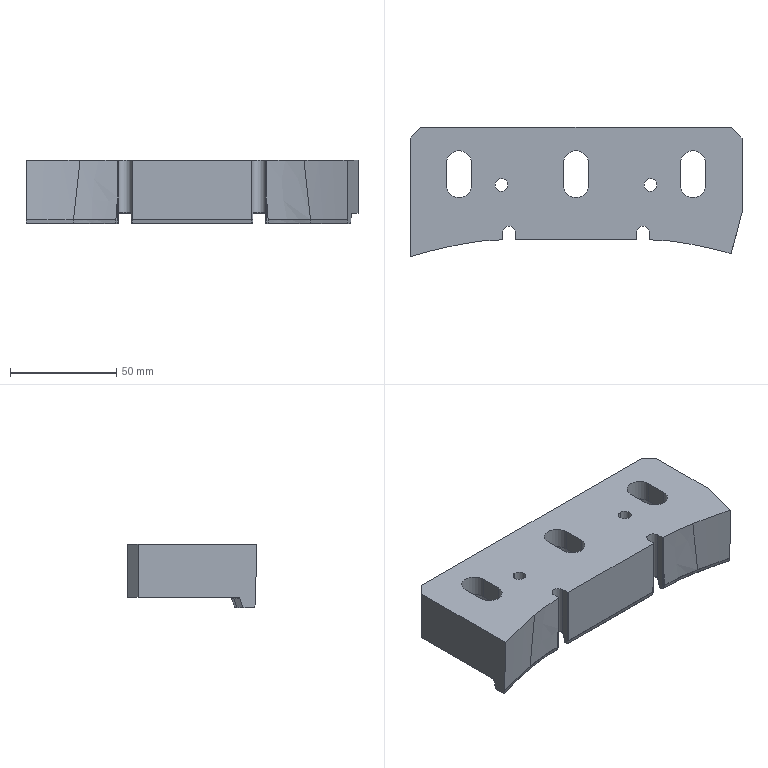NC program | Mastercam | posted with a generic post | part box 156 x 60.706 x 30 mm
Lines 8655 to 9538 of 78092:
N7300 T10 M6
N7310 G0 G90 G17 G54 X-54.9 Y8.053 A0. S1600 M3
N7320 G43 H10 Z50. M8
N7330 Z10.3
N7340 G1 Z.3 F600.
N7350 X-54.4 F1400.
N7360 G3 X-54.1 Y8.353 I0. J.3
N7370 G1 Y13.353 Z.242
N7380 X-54.189 Y13.743 Z.237
N7390 X-54.439 Y14.057 Z.232
N7400 X-54.8 Y14.23 Z.227
N7410 X-55.2 Z.223
N7420 X-55.561 Y14.057 Z.218
N7430 X-55.811 Y13.743 Z.213
N7440 X-55.9 Y13.353 Z.208
N7450 Y3.353 Z.092
N7460 X-55.811 Y2.962 Z.087
N7470 X-55.561 Y2.649 Z.082
N7480 X-55.2 Y2.475 Z.077
N7490 X-54.8 Z.073
N7500 X-54.439 Y2.649 Z.068
N7510 X-54.189 Y2.962 Z.063
N7520 X-54.1 Y3.353 Z.058
N7530 Y8.353 Z0.
N7540 Y13.353 Z-.058
N7550 X-54.189 Y13.743 Z-.063
N7560 X-54.439 Y14.057 Z-.068
N7570 X-54.8 Y14.23 Z-.073
N7580 X-55.2 Z-.077
N7590 X-55.561 Y14.057 Z-.082
N7600 X-55.811 Y13.743 Z-.087
N7610 X-55.9 Y13.353 Z-.092
N7620 Y3.353 Z-.208
N7630 X-55.811 Y2.962 Z-.213
N7640 X-55.561 Y2.649 Z-.218
N7650 X-55.2 Y2.475 Z-.223
N7660 X-54.8 Z-.227
N7670 X-54.439 Y2.649 Z-.232
N7680 X-54.189 Y2.962 Z-.237
N7690 X-54.1 Y3.353 Z-.242
N7700 Y8.353 Z-.3
N7710 Y13.353 Z-.358
N7720 X-54.189 Y13.743 Z-.363
N7730 X-54.439 Y14.057 Z-.368
N7740 X-54.8 Y14.23 Z-.373
N7750 X-55.2 Z-.377
N7760 X-55.561 Y14.057 Z-.382
N7770 X-55.811 Y13.743 Z-.387
N7780 X-55.9 Y13.353 Z-.392
N7790 Y3.353 Z-.508
N7800 X-55.811 Y2.962 Z-.513
N7810 X-55.561 Y2.649 Z-.518
N7820 X-55.2 Y2.475 Z-.523
N7830 X-54.8 Z-.527
N7840 X-54.439 Y2.649 Z-.532
N7850 X-54.189 Y2.962 Z-.537
N7860 X-54.1 Y3.353 Z-.542
N7870 Y8.353 Z-.6
N7880 Y13.353 Z-.658
N7890 X-54.189 Y13.743 Z-.663
N7900 X-54.439 Y14.057 Z-.668
N7910 X-54.8 Y14.23 Z-.673
N7920 X-55.2 Z-.677
N7930 X-55.561 Y14.057 Z-.682
N7940 X-55.811 Y13.743 Z-.687
N7950 X-55.9 Y13.353 Z-.692
N7960 Y3.353 Z-.808
N7970 X-55.811 Y2.962 Z-.813
N7980 X-55.561 Y2.649 Z-.818
N7990 X-55.2 Y2.475 Z-.823
N8000 X-54.8 Z-.827
N8010 X-54.439 Y2.649 Z-.832
N8020 X-54.189 Y2.962 Z-.837
N8030 X-54.1 Y3.353 Z-.842
N8040 Y8.353 Z-.9
N8050 Y13.353 Z-.958
N8060 X-54.189 Y13.743 Z-.963
N8070 X-54.439 Y14.057 Z-.968
N8080 X-54.8 Y14.23 Z-.973
N8090 X-55.2 Z-.977
N8100 X-55.561 Y14.057 Z-.982
N8110 X-55.811 Y13.743 Z-.987
N8120 X-55.9 Y13.353 Z-.992
N8130 Y3.353 Z-1.108
N8140 X-55.811 Y2.962 Z-1.113
N8150 X-55.561 Y2.649 Z-1.118
N8160 X-55.2 Y2.475 Z-1.123
N8170 X-54.8 Z-1.127
N8180 X-54.439 Y2.649 Z-1.132
N8190 X-54.189 Y2.962 Z-1.137
N8200 X-54.1 Y3.353 Z-1.142
N8210 Y8.353 Z-1.2
N8220 Y13.353 Z-1.258
N8230 X-54.189 Y13.743 Z-1.263
N8240 X-54.439 Y14.057 Z-1.268
N8250 X-54.8 Y14.23 Z-1.273
N8260 X-55.2 Z-1.277
N8270 X-55.561 Y14.057 Z-1.282
N8280 X-55.811 Y13.743 Z-1.287
N8290 X-55.9 Y13.353 Z-1.292
N8300 Y3.353 Z-1.408
N8310 X-55.811 Y2.962 Z-1.413
N8320 X-55.561 Y2.649 Z-1.418
N8330 X-55.2 Y2.475 Z-1.423
N8340 X-54.8 Z-1.427
N8350 X-54.439 Y2.649 Z-1.432
N8360 X-54.189 Y2.962 Z-1.437
N8370 X-54.1 Y3.353 Z-1.442
N8380 Y8.353 Z-1.5
N8390 Y13.353 Z-1.558
N8400 X-54.189 Y13.743 Z-1.563
N8410 X-54.439 Y14.057 Z-1.568
N8420 X-54.8 Y14.23 Z-1.573
N8430 X-55.2 Z-1.577
N8440 X-55.561 Y14.057 Z-1.582
N8450 X-55.811 Y13.743 Z-1.587
N8460 X-55.9 Y13.353 Z-1.592
N8470 Y3.353 Z-1.708
N8480 X-55.811 Y2.962 Z-1.713
N8490 X-55.561 Y2.649 Z-1.718
N8500 X-55.2 Y2.475 Z-1.723
N8510 X-54.8 Z-1.727
N8520 X-54.439 Y2.649 Z-1.732
N8530 X-54.189 Y2.962 Z-1.737
N8540 X-54.1 Y3.353 Z-1.742
N8550 Y8.353 Z-1.8
N8560 Y13.353 Z-1.858
N8570 X-54.189 Y13.743 Z-1.863
N8580 X-54.439 Y14.057 Z-1.868
N8590 X-54.8 Y14.23 Z-1.873
N8600 X-55.2 Z-1.877
N8610 X-55.561 Y14.057 Z-1.882
N8620 X-55.811 Y13.743 Z-1.887
N8630 X-55.9 Y13.353 Z-1.892
N8640 Y3.353 Z-2.008
N8650 X-55.811 Y2.962 Z-2.013
N8660 X-55.561 Y2.649 Z-2.018
N8670 X-55.2 Y2.475 Z-2.023
N8680 X-54.8 Z-2.027
N8690 X-54.439 Y2.649 Z-2.032
N8700 X-54.189 Y2.962 Z-2.037
N8710 X-54.1 Y3.353 Z-2.042
N8720 Y8.353 Z-2.1
N8730 Y13.353 Z-2.158
N8740 X-54.189 Y13.743 Z-2.163
N8750 X-54.439 Y14.057 Z-2.168
N8760 X-54.8 Y14.23 Z-2.173
N8770 X-55.2 Z-2.177
N8780 X-55.561 Y14.057 Z-2.182
N8790 X-55.811 Y13.743 Z-2.187
N8800 X-55.9 Y13.353 Z-2.192
N8810 Y3.353 Z-2.308
N8820 X-55.811 Y2.962 Z-2.313
N8830 X-55.561 Y2.649 Z-2.318
N8840 X-55.2 Y2.475 Z-2.323
N8850 X-54.8 Z-2.327
N8860 X-54.439 Y2.649 Z-2.332
N8870 X-54.189 Y2.962 Z-2.337
N8880 X-54.1 Y3.353 Z-2.342
N8890 Y8.353 Z-2.4
N8900 Y13.353 Z-2.458
N8910 X-54.189 Y13.743 Z-2.463
N8920 X-54.439 Y14.057 Z-2.468
N8930 X-54.8 Y14.23 Z-2.473
N8940 X-55.2 Z-2.477
N8950 X-55.561 Y14.057 Z-2.482
N8960 X-55.811 Y13.743 Z-2.487
N8970 X-55.9 Y13.353 Z-2.492
N8980 Y3.353 Z-2.608
N8990 X-55.811 Y2.962 Z-2.613
N9000 X-55.561 Y2.649 Z-2.618
N9010 X-55.2 Y2.475 Z-2.623
N9020 X-54.8 Z-2.627
N9030 X-54.439 Y2.649 Z-2.632
N9040 X-54.189 Y2.962 Z-2.637
N9050 X-54.1 Y3.353 Z-2.642
N9060 Y8.353 Z-2.7
N9070 Y13.353 Z-2.758
N9080 X-54.189 Y13.743 Z-2.763
N9090 X-54.439 Y14.057 Z-2.768
N9100 X-54.8 Y14.23 Z-2.773
N9110 X-55.2 Z-2.777
N9120 X-55.561 Y14.057 Z-2.782
N9130 X-55.811 Y13.743 Z-2.787
N9140 X-55.9 Y13.353 Z-2.792
N9150 Y3.353 Z-2.908
N9160 X-55.811 Y2.962 Z-2.913
N9170 X-55.561 Y2.649 Z-2.918
N9180 X-55.2 Y2.475 Z-2.923
N9190 X-54.8 Z-2.927
N9200 X-54.439 Y2.649 Z-2.932
N9210 X-54.189 Y2.962 Z-2.937
N9220 X-54.1 Y3.353 Z-2.942
N9230 Y8.353 Z-3.
N9240 Y13.353 Z-3.058
N9250 X-54.189 Y13.743 Z-3.063
N9260 X-54.439 Y14.057 Z-3.068
N9270 X-54.8 Y14.23 Z-3.073
N9280 X-55.2 Z-3.077
N9290 X-55.561 Y14.057 Z-3.082
N9300 X-55.811 Y13.743 Z-3.087
N9310 X-55.9 Y13.353 Z-3.092
N9320 Y3.353 Z-3.208
N9330 X-55.811 Y2.962 Z-3.213
N9340 X-55.561 Y2.649 Z-3.218
N9350 X-55.2 Y2.475 Z-3.223
N9360 X-54.8 Z-3.227
N9370 X-54.439 Y2.649 Z-3.232
N9380 X-54.189 Y2.962 Z-3.237
N9390 X-54.1 Y3.353 Z-3.242
N9400 Y8.353 Z-3.3
N9410 Y13.353 Z-3.358
N9420 X-54.189 Y13.743 Z-3.363
N9430 X-54.439 Y14.057 Z-3.368
N9440 X-54.8 Y14.23 Z-3.373
N9450 X-55.2 Z-3.377
N9460 X-55.561 Y14.057 Z-3.382
N9470 X-55.811 Y13.743 Z-3.387
N9480 X-55.9 Y13.353 Z-3.392
N9490 Y3.353 Z-3.508
N9500 X-55.811 Y2.962 Z-3.513
N9510 X-55.561 Y2.649 Z-3.518
N9520 X-55.2 Y2.475 Z-3.523
N9530 X-54.8 Z-3.527
N9540 X-54.439 Y2.649 Z-3.532
N9550 X-54.189 Y2.962 Z-3.537
N9560 X-54.1 Y3.353 Z-3.542
N9570 Y8.353 Z-3.6
N9580 Y13.353 Z-3.658
N9590 X-54.189 Y13.743 Z-3.663
N9600 X-54.439 Y14.057 Z-3.668
N9610 X-54.8 Y14.23 Z-3.673
N9620 X-55.2 Z-3.677
N9630 X-55.561 Y14.057 Z-3.682
N9640 X-55.811 Y13.743 Z-3.687
N9650 X-55.9 Y13.353 Z-3.692
N9660 Y3.353 Z-3.808
N9670 X-55.811 Y2.962 Z-3.813
N9680 X-55.561 Y2.649 Z-3.818
N9690 X-55.2 Y2.475 Z-3.823
N9700 X-54.8 Z-3.827
N9710 X-54.439 Y2.649 Z-3.832
N9720 X-54.189 Y2.962 Z-3.837
N9730 X-54.1 Y3.353 Z-3.842
N9740 Y8.353 Z-3.9
N9750 Y13.353 Z-3.958
N9760 X-54.189 Y13.743 Z-3.963
N9770 X-54.439 Y14.057 Z-3.968
N9780 X-54.8 Y14.23 Z-3.973
N9790 X-55.2 Z-3.977
N9800 X-55.561 Y14.057 Z-3.982
N9810 X-55.811 Y13.743 Z-3.987
N9820 X-55.9 Y13.353 Z-3.992
N9830 Y3.353 Z-4.108
N9840 X-55.811 Y2.962 Z-4.113
N9850 X-55.561 Y2.649 Z-4.118
N9860 X-55.2 Y2.475 Z-4.123
N9870 X-54.8 Z-4.127
N9880 X-54.439 Y2.649 Z-4.132
N9890 X-54.189 Y2.962 Z-4.137
N9900 X-54.1 Y3.353 Z-4.142
N9910 Y8.353 Z-4.2
N9920 Y13.353 Z-4.258
N9930 X-54.189 Y13.743 Z-4.263
N9940 X-54.439 Y14.057 Z-4.268
N9950 X-54.8 Y14.23 Z-4.273
N9960 X-55.2 Z-4.277
N9970 X-55.561 Y14.057 Z-4.282
N9980 X-55.811 Y13.743 Z-4.287
N9990 X-55.9 Y13.353 Z-4.292
N100 Y3.353 Z-4.408
N110 X-55.811 Y2.962 Z-4.413
N120 X-55.561 Y2.649 Z-4.418
N130 X-55.2 Y2.475 Z-4.423
N140 X-54.8 Z-4.427
N150 X-54.439 Y2.649 Z-4.432
N160 X-54.189 Y2.962 Z-4.437
N170 X-54.1 Y3.353 Z-4.442
N180 Y8.353 Z-4.5
N190 Y13.353 Z-4.558
N200 X-54.189 Y13.743 Z-4.563
N210 X-54.439 Y14.057 Z-4.568
N220 X-54.8 Y14.23 Z-4.573
N230 X-55.2 Z-4.577
N240 X-55.561 Y14.057 Z-4.582
N250 X-55.811 Y13.743 Z-4.587
N260 X-55.9 Y13.353 Z-4.592
N270 Y3.353 Z-4.708
N280 X-55.811 Y2.962 Z-4.713
N290 X-55.561 Y2.649 Z-4.718
N300 X-55.2 Y2.475 Z-4.723
N310 X-54.8 Z-4.727
N320 X-54.439 Y2.649 Z-4.732
N330 X-54.189 Y2.962 Z-4.737
N340 X-54.1 Y3.353 Z-4.742
N350 Y8.353 Z-4.8
N360 Y13.353 Z-4.858
N370 X-54.189 Y13.743 Z-4.863
N380 X-54.439 Y14.057 Z-4.868
N390 X-54.8 Y14.23 Z-4.873
N400 X-55.2 Z-4.877
N410 X-55.561 Y14.057 Z-4.882
N420 X-55.811 Y13.743 Z-4.887
N430 X-55.9 Y13.353 Z-4.892
N440 Y3.353 Z-5.008
N450 X-55.811 Y2.962 Z-5.013
N460 X-55.561 Y2.649 Z-5.018
N470 X-55.2 Y2.475 Z-5.023
N480 X-54.8 Z-5.027
N490 X-54.439 Y2.649 Z-5.032
N500 X-54.189 Y2.962 Z-5.037
N510 X-54.1 Y3.353 Z-5.042
N520 Y8.353 Z-5.1
N530 Y13.353 Z-5.158
N540 X-54.189 Y13.743 Z-5.163
N550 X-54.439 Y14.057 Z-5.168
N560 X-54.8 Y14.23 Z-5.173
N570 X-55.2 Z-5.177
N580 X-55.561 Y14.057 Z-5.182
N590 X-55.811 Y13.743 Z-5.187
N600 X-55.9 Y13.353 Z-5.192
N610 Y3.353 Z-5.308
N620 X-55.811 Y2.962 Z-5.313
N630 X-55.561 Y2.649 Z-5.318
N640 X-55.2 Y2.475 Z-5.323
N650 X-54.8 Z-5.327
N660 X-54.439 Y2.649 Z-5.332
N670 X-54.189 Y2.962 Z-5.337
N680 X-54.1 Y3.353 Z-5.342
N690 Y8.353 Z-5.4
N700 Y13.353 Z-5.458
N710 X-54.189 Y13.743 Z-5.463
N720 X-54.439 Y14.057 Z-5.468
N730 X-54.8 Y14.23 Z-5.473
N740 X-55.2 Z-5.477
N750 X-55.561 Y14.057 Z-5.482
N760 X-55.811 Y13.743 Z-5.487
N770 X-55.9 Y13.353 Z-5.492
N780 Y3.353 Z-5.608
N790 X-55.811 Y2.962 Z-5.613
N800 X-55.561 Y2.649 Z-5.618
N810 X-55.2 Y2.475 Z-5.623
N820 X-54.8 Z-5.627
N830 X-54.439 Y2.649 Z-5.632
N840 X-54.189 Y2.962 Z-5.637
N850 X-54.1 Y3.353 Z-5.642
N860 Y8.353 Z-5.7
N870 Y13.353 Z-5.758
N880 X-54.189 Y13.743 Z-5.763
N890 X-54.439 Y14.057 Z-5.768
N900 X-54.8 Y14.23 Z-5.773
N910 X-55.2 Z-5.777
N920 X-55.561 Y14.057 Z-5.782
N930 X-55.811 Y13.743 Z-5.787
N940 X-55.9 Y13.353 Z-5.792
N950 Y3.353 Z-5.908
N960 X-55.811 Y2.962 Z-5.913
N970 X-55.561 Y2.649 Z-5.918
N980 X-55.2 Y2.475 Z-5.923
N990 X-54.8 Z-5.927
N1000 X-54.439 Y2.649 Z-5.932
N1010 X-54.189 Y2.962 Z-5.937
N1020 X-54.1 Y3.353 Z-5.942
N1030 Y8.353 Z-6.
N1040 Y13.353 Z-6.058
N1050 X-54.189 Y13.743 Z-6.063
N1060 X-54.439 Y14.057 Z-6.068
N1070 X-54.8 Y14.23 Z-6.073
N1080 X-55.2 Z-6.077
N1090 X-55.561 Y14.057 Z-6.082
N1100 X-55.811 Y13.743 Z-6.087
N1110 X-55.9 Y13.353 Z-6.092
N1120 Y3.353 Z-6.208
N1130 X-55.811 Y2.962 Z-6.213
N1140 X-55.561 Y2.649 Z-6.218
N1150 X-55.2 Y2.475 Z-6.223
N1160 X-54.8 Z-6.227
N1170 X-54.439 Y2.649 Z-6.232
N1180 X-54.189 Y2.962 Z-6.237
N1190 X-54.1 Y3.353 Z-6.242
N1200 Y8.353 Z-6.3
N1210 Y13.353 Z-6.358
N1220 X-54.189 Y13.743 Z-6.363
N1230 X-54.439 Y14.057 Z-6.368
N1240 X-54.8 Y14.23 Z-6.373
N1250 X-55.2 Z-6.377
N1260 X-55.561 Y14.057 Z-6.382
N1270 X-55.811 Y13.743 Z-6.387
N1280 X-55.9 Y13.353 Z-6.392
N1290 Y3.353 Z-6.508
N1300 X-55.811 Y2.962 Z-6.513
N1310 X-55.561 Y2.649 Z-6.518
N1320 X-55.2 Y2.475 Z-6.523
N1330 X-54.8 Z-6.527
N1340 X-54.439 Y2.649 Z-6.532
N1350 X-54.189 Y2.962 Z-6.537
N1360 X-54.1 Y3.353 Z-6.542
N1370 Y8.353 Z-6.6
N1380 Y13.353 Z-6.658
N1390 X-54.189 Y13.743 Z-6.663
N1400 X-54.439 Y14.057 Z-6.668
N1410 X-54.8 Y14.23 Z-6.673
N1420 X-55.2 Z-6.677
N1430 X-55.561 Y14.057 Z-6.682
N1440 X-55.811 Y13.743 Z-6.687
N1450 X-55.9 Y13.353 Z-6.692
N1460 Y3.353 Z-6.808
N1470 X-55.811 Y2.962 Z-6.813
N1480 X-55.561 Y2.649 Z-6.818
N1490 X-55.2 Y2.475 Z-6.823
N1500 X-54.8 Z-6.827
N1510 X-54.439 Y2.649 Z-6.832
N1520 X-54.189 Y2.962 Z-6.837
N1530 X-54.1 Y3.353 Z-6.842
N1540 Y8.353 Z-6.9
N1550 Y13.353 Z-6.958
N1560 X-54.189 Y13.743 Z-6.963
N1570 X-54.439 Y14.057 Z-6.968
N1580 X-54.8 Y14.23 Z-6.973
N1590 X-55.2 Z-6.977
N1600 X-55.561 Y14.057 Z-6.982
N1610 X-55.811 Y13.743 Z-6.987
N1620 X-55.9 Y13.353 Z-6.992
N1630 Y3.353 Z-7.108
N1640 X-55.811 Y2.962 Z-7.113
N1650 X-55.561 Y2.649 Z-7.118
N1660 X-55.2 Y2.475 Z-7.123
N1670 X-54.8 Z-7.127
N1680 X-54.439 Y2.649 Z-7.132
N1690 X-54.189 Y2.962 Z-7.137
N1700 X-54.1 Y3.353 Z-7.142
N1710 Y8.353 Z-7.2
N1720 Y13.353 Z-7.258
N1730 X-54.189 Y13.743 Z-7.263
N1740 X-54.439 Y14.057 Z-7.268
N1750 X-54.8 Y14.23 Z-7.273
N1760 X-55.2 Z-7.277
N1770 X-55.561 Y14.057 Z-7.282
N1780 X-55.811 Y13.743 Z-7.287
N1790 X-55.9 Y13.353 Z-7.292
N1800 Y3.353 Z-7.408
N1810 X-55.811 Y2.962 Z-7.413
N1820 X-55.561 Y2.649 Z-7.418
N1830 X-55.2 Y2.475 Z-7.423
N1840 X-54.8 Z-7.427
N1850 X-54.439 Y2.649 Z-7.432
N1860 X-54.189 Y2.962 Z-7.437
N1870 X-54.1 Y3.353 Z-7.442
N1880 Y8.353 Z-7.5
N1890 Y13.353 Z-7.558
N1900 X-54.189 Y13.743 Z-7.563
N1910 X-54.439 Y14.057 Z-7.568
N1920 X-54.8 Y14.23 Z-7.573
N1930 X-55.2 Z-7.577
N1940 X-55.561 Y14.057 Z-7.582
N1950 X-55.811 Y13.743 Z-7.587
N1960 X-55.9 Y13.353 Z-7.592
N1970 Y3.353 Z-7.708
N1980 X-55.811 Y2.962 Z-7.713
N1990 X-55.561 Y2.649 Z-7.718
N2000 X-55.2 Y2.475 Z-7.723
N2010 X-54.8 Z-7.727
N2020 X-54.439 Y2.649 Z-7.732
N2030 X-54.189 Y2.962 Z-7.737
N2040 X-54.1 Y3.353 Z-7.742
N2050 Y8.353 Z-7.8
N2060 Y13.353 Z-7.858
N2070 X-54.189 Y13.743 Z-7.863
N2080 X-54.439 Y14.057 Z-7.868
N2090 X-54.8 Y14.23 Z-7.873
N2100 X-55.2 Z-7.877
N2110 X-55.561 Y14.057 Z-7.882
N2120 X-55.811 Y13.743 Z-7.887
N2130 X-55.9 Y13.353 Z-7.892
N2140 Y3.353 Z-8.008
N2150 X-55.811 Y2.962 Z-8.013
N2160 X-55.561 Y2.649 Z-8.018
N2170 X-55.2 Y2.475 Z-8.023
N2180 X-54.8 Z-8.027
N2190 X-54.439 Y2.649 Z-8.032
N2200 X-54.189 Y2.962 Z-8.037
N2210 X-54.1 Y3.353 Z-8.042
N2220 Y8.353 Z-8.1
N2230 Y13.353 Z-8.158
N2240 X-54.189 Y13.743 Z-8.163
N2250 X-54.439 Y14.057 Z-8.168
N2260 X-54.8 Y14.23 Z-8.173
N2270 X-55.2 Z-8.177
N2280 X-55.561 Y14.057 Z-8.182
N2290 X-55.811 Y13.743 Z-8.187
N2300 X-55.9 Y13.353 Z-8.192
N2310 Y3.353 Z-8.308
N2320 X-55.811 Y2.962 Z-8.313
N2330 X-55.561 Y2.649 Z-8.318
N2340 X-55.2 Y2.475 Z-8.323
N2350 X-54.8 Z-8.327
N2360 X-54.439 Y2.649 Z-8.332
N2370 X-54.189 Y2.962 Z-8.337
N2380 X-54.1 Y3.353 Z-8.342
N2390 Y8.353 Z-8.4
N2400 Y13.353 Z-8.458
N2410 X-54.189 Y13.743 Z-8.463
N2420 X-54.439 Y14.057 Z-8.468
N2430 X-54.8 Y14.23 Z-8.473
N2440 X-55.2 Z-8.477
N2450 X-55.561 Y14.057 Z-8.482
N2460 X-55.811 Y13.743 Z-8.487
N2470 X-55.9 Y13.353 Z-8.492
N2480 Y3.353 Z-8.608
N2490 X-55.811 Y2.962 Z-8.613
N2500 X-55.561 Y2.649 Z-8.618
N2510 X-55.2 Y2.475 Z-8.623
N2520 X-54.8 Z-8.627
N2530 X-54.439 Y2.649 Z-8.632
N2540 X-54.189 Y2.962 Z-8.637
N2550 X-54.1 Y3.353 Z-8.642
N2560 Y8.353 Z-8.7
N2570 Y13.353 Z-8.758
N2580 X-54.189 Y13.743 Z-8.763
N2590 X-54.439 Y14.057 Z-8.768
N2600 X-54.8 Y14.23 Z-8.773
N2610 X-55.2 Z-8.777
N2620 X-55.561 Y14.057 Z-8.782
N2630 X-55.811 Y13.743 Z-8.787
N2640 X-55.9 Y13.353 Z-8.792
N2650 Y3.353 Z-8.908
N2660 X-55.811 Y2.962 Z-8.913
N2670 X-55.561 Y2.649 Z-8.918
N2680 X-55.2 Y2.475 Z-8.923
N2690 X-54.8 Z-8.927
N2700 X-54.439 Y2.649 Z-8.932
N2710 X-54.189 Y2.962 Z-8.937
N2720 X-54.1 Y3.353 Z-8.942
N2730 Y8.353 Z-9.
N2740 Y13.353 Z-9.058
N2750 X-54.189 Y13.743 Z-9.063
N2760 X-54.439 Y14.057 Z-9.068
N2770 X-54.8 Y14.23 Z-9.073
N2780 X-55.2 Z-9.077
N2790 X-55.561 Y14.057 Z-9.082
N2800 X-55.811 Y13.743 Z-9.087
N2810 X-55.9 Y13.353 Z-9.092
N2820 Y3.353 Z-9.208
N2830 X-55.811 Y2.962 Z-9.213
N2840 X-55.561 Y2.649 Z-9.218
N2850 X-55.2 Y2.475 Z-9.223
N2860 X-54.8 Z-9.227
N2870 X-54.439 Y2.649 Z-9.232
N2880 X-54.189 Y2.962 Z-9.237
N2890 X-54.1 Y3.353 Z-9.242
N2900 Y8.353 Z-9.3
N2910 Y13.353 Z-9.358
N2920 X-54.189 Y13.743 Z-9.363
N2930 X-54.439 Y14.057 Z-9.368
N2940 X-54.8 Y14.23 Z-9.373
N2950 X-55.2 Z-9.377
N2960 X-55.561 Y14.057 Z-9.382
N2970 X-55.811 Y13.743 Z-9.387
N2980 X-55.9 Y13.353 Z-9.392
N2990 Y3.353 Z-9.508
N3000 X-55.811 Y2.962 Z-9.513
N3010 X-55.561 Y2.649 Z-9.518
N3020 X-55.2 Y2.475 Z-9.523
N3030 X-54.8 Z-9.527
N3040 X-54.439 Y2.649 Z-9.532
N3050 X-54.189 Y2.962 Z-9.537
N3060 X-54.1 Y3.353 Z-9.542
N3070 Y8.353 Z-9.6
N3080 Y13.353 Z-9.658
N3090 X-54.189 Y13.743 Z-9.663
N3100 X-54.439 Y14.057 Z-9.668
N3110 X-54.8 Y14.23 Z-9.673
N3120 X-55.2 Z-9.677
N3130 X-55.561 Y14.057 Z-9.682
N3140 X-55.811 Y13.743 Z-9.687
N3150 X-55.9 Y13.353 Z-9.692
N3160 Y3.353 Z-9.808
N3170 X-55.811 Y2.962 Z-9.813
N3180 X-55.561 Y2.649 Z-9.818
N3190 X-55.2 Y2.475 Z-9.823
N3200 X-54.8 Z-9.827
N3210 X-54.439 Y2.649 Z-9.832
N3220 X-54.189 Y2.962 Z-9.837
N3230 X-54.1 Y3.353 Z-9.842
N3240 Y8.353 Z-9.9
N3250 Y13.353 Z-9.958
N3260 X-54.189 Y13.743 Z-9.963
N3270 X-54.439 Y14.057 Z-9.968
N3280 X-54.8 Y14.23 Z-9.973
N3290 X-55.2 Z-9.977
N3300 X-55.561 Y14.057 Z-9.982
N3310 X-55.811 Y13.743 Z-9.987
N3320 X-55.9 Y13.353 Z-9.992
N3330 Y3.353 Z-10.108
N3340 X-55.811 Y2.962 Z-10.113
N3350 X-55.561 Y2.649 Z-10.118
N3360 X-55.2 Y2.475 Z-10.123
N3370 X-54.8 Z-10.127
N3380 X-54.439 Y2.649 Z-10.132
N3390 X-54.189 Y2.962 Z-10.137
N3400 X-54.1 Y3.353 Z-10.142
N3410 Y8.353 Z-10.2
N3420 Y13.353 Z-10.258
N3430 X-54.189 Y13.743 Z-10.263
N3440 X-54.439 Y14.057 Z-10.268
N3450 X-54.8 Y14.23 Z-10.273
N3460 X-55.2 Z-10.277
N3470 X-55.561 Y14.057 Z-10.282
N3480 X-55.811 Y13.743 Z-10.287
N3490 X-55.9 Y13.353 Z-10.292
N3500 Y3.353 Z-10.408
N3510 X-55.811 Y2.962 Z-10.413
N3520 X-55.561 Y2.649 Z-10.418
N3530 X-55.2 Y2.475 Z-10.423
N3540 X-54.8 Z-10.427
N3550 X-54.439 Y2.649 Z-10.432
N3560 X-54.189 Y2.962 Z-10.437
N3570 X-54.1 Y3.353 Z-10.442
N3580 Y8.353 Z-10.5
N3590 Y13.353 Z-10.558
N3600 X-54.189 Y13.743 Z-10.563
N3610 X-54.439 Y14.057 Z-10.568
N3620 X-54.8 Y14.23 Z-10.573
N3630 X-55.2 Z-10.577
N3640 X-55.561 Y14.057 Z-10.582
N3650 X-55.811 Y13.743 Z-10.587
N3660 X-55.9 Y13.353 Z-10.592
N3670 Y3.353 Z-10.708
N3680 X-55.811 Y2.962 Z-10.713
N3690 X-55.561 Y2.649 Z-10.718
N3700 X-55.2 Y2.475 Z-10.723
N3710 X-54.8 Z-10.727
N3720 X-54.439 Y2.649 Z-10.732
N3730 X-54.189 Y2.962 Z-10.737
N3740 X-54.1 Y3.353 Z-10.742
N3750 Y8.353 Z-10.8
N3760 Y13.353 Z-10.858
N3770 X-54.189 Y13.743 Z-10.863
N3780 X-54.439 Y14.057 Z-10.868
N3790 X-54.8 Y14.23 Z-10.873
N3800 X-55.2 Z-10.877
N3810 X-55.561 Y14.057 Z-10.882
N3820 X-55.811 Y13.743 Z-10.887
N3830 X-55.9 Y13.353 Z-10.892
N3840 Y3.353 Z-11.008
N3850 X-55.811 Y2.962 Z-11.013
N3860 X-55.561 Y2.649 Z-11.018
N3870 X-55.2 Y2.475 Z-11.023
N3880 X-54.8 Z-11.027
N3890 X-54.439 Y2.649 Z-11.032
N3900 X-54.189 Y2.962 Z-11.037
N3910 X-54.1 Y3.353 Z-11.042
N3920 Y8.353 Z-11.1
N3930 Y13.353 Z-11.158
N3940 X-54.189 Y13.743 Z-11.163
N3950 X-54.439 Y14.057 Z-11.168
N3960 X-54.8 Y14.23 Z-11.173
N3970 X-55.2 Z-11.177
N3980 X-55.561 Y14.057 Z-11.182
N3990 X-55.811 Y13.743 Z-11.187
N4000 X-55.9 Y13.353 Z-11.192
N4010 Y3.353 Z-11.308
N4020 X-55.811 Y2.962 Z-11.313
N4030 X-55.561 Y2.649 Z-11.318
N4040 X-55.2 Y2.475 Z-11.323
N4050 X-54.8 Z-11.327
N4060 X-54.439 Y2.649 Z-11.332
N4070 X-54.189 Y2.962 Z-11.337
N4080 X-54.1 Y3.353 Z-11.342
N4090 Y8.353 Z-11.4
N4100 Y13.353 Z-11.458
N4110 X-54.189 Y13.743 Z-11.463
N4120 X-54.439 Y14.057 Z-11.468
N4130 X-54.8 Y14.23 Z-11.473
N4140 X-55.2 Z-11.477
N4150 X-55.561 Y14.057 Z-11.482
N4160 X-55.811 Y13.743 Z-11.487
N4170 X-55.9 Y13.353 Z-11.492
N4180 Y3.353 Z-11.608
N4190 X-55.811 Y2.962 Z-11.613
N4200 X-55.561 Y2.649 Z-11.618
N4210 X-55.2 Y2.475 Z-11.623
N4220 X-54.8 Z-11.627
N4230 X-54.439 Y2.649 Z-11.632
N4240 X-54.189 Y2.962 Z-11.637
N4250 X-54.1 Y3.353 Z-11.642
N4260 Y8.353 Z-11.7
N4270 Y13.353 Z-11.758
N4280 X-54.189 Y13.743 Z-11.763
N4290 X-54.439 Y14.057 Z-11.768
N4300 X-54.8 Y14.23 Z-11.773
N4310 X-55.2 Z-11.777
N4320 X-55.561 Y14.057 Z-11.782
N4330 X-55.811 Y13.743 Z-11.787
N4340 X-55.9 Y13.353 Z-11.792
N4350 Y3.353 Z-11.908
N4360 X-55.811 Y2.962 Z-11.913
N4370 X-55.561 Y2.649 Z-11.918
N4380 X-55.2 Y2.475 Z-11.923
N4390 X-54.8 Z-11.927
N4400 X-54.439 Y2.649 Z-11.932
N4410 X-54.189 Y2.962 Z-11.937
N4420 X-54.1 Y3.353 Z-11.942
N4430 Y8.353 Z-12.
N4440 Y13.353 Z-12.058
N4450 X-54.189 Y13.743 Z-12.063
N4460 X-54.439 Y14.057 Z-12.068
N4470 X-54.8 Y14.23 Z-12.073
N4480 X-55.2 Z-12.077
N4490 X-55.561 Y14.057 Z-12.082
N4500 X-55.811 Y13.743 Z-12.087
N4510 X-55.9 Y13.353 Z-12.092
N4520 Y3.353 Z-12.208
N4530 X-55.811 Y2.962 Z-12.213
N4540 X-55.561 Y2.649 Z-12.218
N4550 X-55.2 Y2.475 Z-12.223
N4560 X-54.8 Z-12.227
N4570 X-54.439 Y2.649 Z-12.232
N4580 X-54.189 Y2.962 Z-12.237
N4590 X-54.1 Y3.353 Z-12.242
N4600 Y8.353 Z-12.3
N4610 Y13.353 Z-12.358
N4620 X-54.189 Y13.743 Z-12.363
N4630 X-54.439 Y14.057 Z-12.368
N4640 X-54.8 Y14.23 Z-12.373
N4650 X-55.2 Z-12.377
N4660 X-55.561 Y14.057 Z-12.382
N4670 X-55.811 Y13.743 Z-12.387
N4680 X-55.9 Y13.353 Z-12.392
N4690 Y3.353 Z-12.508
N4700 X-55.811 Y2.962 Z-12.513
N4710 X-55.561 Y2.649 Z-12.518
N4720 X-55.2 Y2.475 Z-12.523
N4730 X-54.8 Z-12.527
N4740 X-54.439 Y2.649 Z-12.532
N4750 X-54.189 Y2.962 Z-12.537
N4760 X-54.1 Y3.353 Z-12.542
N4770 Y8.353 Z-12.6
N4780 Y13.353 Z-12.658
N4790 X-54.189 Y13.743 Z-12.663
N4800 X-54.439 Y14.057 Z-12.668
N4810 X-54.8 Y14.23 Z-12.673
N4820 X-55.2 Z-12.677
N4830 X-55.561 Y14.057 Z-12.682
N4840 X-55.811 Y13.743 Z-12.687
N4850 X-55.9 Y13.353 Z-12.692
N4860 Y3.353 Z-12.808
N4870 X-55.811 Y2.962 Z-12.813
N4880 X-55.561 Y2.649 Z-12.818
N4890 X-55.2 Y2.475 Z-12.823
N4900 X-54.8 Z-12.827
N4910 X-54.439 Y2.649 Z-12.832
N4920 X-54.189 Y2.962 Z-12.837
N4930 X-54.1 Y3.353 Z-12.842
N4940 Y8.353 Z-12.9
N4950 Y13.353 Z-12.958
N4960 X-54.189 Y13.743 Z-12.963
N4970 X-54.439 Y14.057 Z-12.968
N4980 X-54.8 Y14.23 Z-12.973
N4990 X-55.2 Z-12.977
N5000 X-55.561 Y14.057 Z-12.982
N5010 X-55.811 Y13.743 Z-12.987
N5020 X-55.9 Y13.353 Z-12.992
N5030 Y3.353 Z-13.108
N5040 X-55.811 Y2.962 Z-13.113
N5050 X-55.561 Y2.649 Z-13.118
N5060 X-55.2 Y2.475 Z-13.123
N5070 X-54.8 Z-13.127
N5080 X-54.439 Y2.649 Z-13.132
N5090 X-54.189 Y2.962 Z-13.137
N5100 X-54.1 Y3.353 Z-13.142
N5110 Y8.353 Z-13.2
N5120 Y13.353 Z-13.258
N5130 X-54.189 Y13.743 Z-13.263
N5140 X-54.439 Y14.057 Z-13.268
N5150 X-54.8 Y14.23 Z-13.273
N5160 X-55.2 Z-13.277
N5170 X-55.561 Y14.057 Z-13.282
N5180 X-55.811 Y13.743 Z-13.287
N5190 X-55.9 Y13.353 Z-13.292
N5200 Y3.353 Z-13.408
N5210 X-55.811 Y2.962 Z-13.413
N5220 X-55.561 Y2.649 Z-13.418
N5230 X-55.2 Y2.475 Z-13.423
N5240 X-54.8 Z-13.427
N5250 X-54.439 Y2.649 Z-13.432
N5260 X-54.189 Y2.962 Z-13.437
N5270 X-54.1 Y3.353 Z-13.442
N5280 Y8.353 Z-13.5
N5290 Y13.353 Z-13.558
N5300 X-54.189 Y13.743 Z-13.563
N5310 X-54.439 Y14.057 Z-13.568
N5320 X-54.8 Y14.23 Z-13.573
N5330 X-55.2 Z-13.577
N5340 X-55.561 Y14.057 Z-13.582
N5350 X-55.811 Y13.743 Z-13.587
N5360 X-55.9 Y13.353 Z-13.592
N5370 Y3.353 Z-13.708
N5380 X-55.811 Y2.962 Z-13.713
N5390 X-55.561 Y2.649 Z-13.718
N5400 X-55.2 Y2.475 Z-13.723
N5410 X-54.8 Z-13.727
N5420 X-54.439 Y2.649 Z-13.732
N5430 X-54.189 Y2.962 Z-13.737
N5440 X-54.1 Y3.353 Z-13.742
N5450 Y8.353 Z-13.8
N5460 Y13.353 Z-13.858
N5470 X-54.189 Y13.743 Z-13.863
N5480 X-54.439 Y14.057 Z-13.868
N5490 X-54.8 Y14.23 Z-13.873
N5500 X-55.2 Z-13.877
N5510 X-55.561 Y14.057 Z-13.882
N5520 X-55.811 Y13.743 Z-13.887
N5530 X-55.9 Y13.353 Z-13.892
N5540 Y3.353 Z-14.008
N5550 X-55.811 Y2.962 Z-14.013
N5560 X-55.561 Y2.649 Z-14.018
N5570 X-55.2 Y2.475 Z-14.023
N5580 X-54.8 Z-14.027
N5590 X-54.439 Y2.649 Z-14.032
N5600 X-54.189 Y2.962 Z-14.037
N5610 X-54.1 Y3.353 Z-14.042
N5620 Y8.353 Z-14.1
N5630 Y13.353 Z-14.158
N5640 X-54.189 Y13.743 Z-14.163
N5650 X-54.439 Y14.057 Z-14.168
N5660 X-54.8 Y14.23 Z-14.173
N5670 X-55.2 Z-14.177
N5680 X-55.561 Y14.057 Z-14.182
N5690 X-55.811 Y13.743 Z-14.187
N5700 X-55.9 Y13.353 Z-14.192
N5710 Y3.353 Z-14.308
N5720 X-55.811 Y2.962 Z-14.313
N5730 X-55.561 Y2.649 Z-14.318
N5740 X-55.2 Y2.475 Z-14.323
N5750 X-54.8 Z-14.327
N5760 X-54.439 Y2.649 Z-14.332
N5770 X-54.189 Y2.962 Z-14.337
N5780 X-54.1 Y3.353 Z-14.342
N5790 Y8.353 Z-14.4
N5800 Y13.353 Z-14.458
N5810 X-54.189 Y13.743 Z-14.463
N5820 X-54.439 Y14.057 Z-14.468
N5830 X-54.8 Y14.23 Z-14.473
N5840 X-55.2 Z-14.477
N5850 X-55.561 Y14.057 Z-14.482
N5860 X-55.811 Y13.743 Z-14.487
N5870 X-55.9 Y13.353 Z-14.492
N5880 Y3.353 Z-14.608
N5890 X-55.811 Y2.962 Z-14.613
N5900 X-55.561 Y2.649 Z-14.618
N5910 X-55.2 Y2.475 Z-14.623
N5920 X-54.8 Z-14.627
N5930 X-54.439 Y2.649 Z-14.632
N5940 X-54.189 Y2.962 Z-14.637
N5950 X-54.1 Y3.353 Z-14.642
N5960 Y8.353 Z-14.7
N5970 Y13.353 Z-14.758
N5980 X-54.189 Y13.743 Z-14.763
N5990 X-54.439 Y14.057 Z-14.768
N6000 X-54.8 Y14.23 Z-14.773
N6010 X-55.2 Z-14.777
N6020 X-55.561 Y14.057 Z-14.782
N6030 X-55.811 Y13.743 Z-14.787
N6040 X-55.9 Y13.353 Z-14.792
N6050 Y3.353 Z-14.908
N6060 X-55.811 Y2.962 Z-14.913
N6070 X-55.561 Y2.649 Z-14.918
N6080 X-55.2 Y2.475 Z-14.923
N6090 X-54.8 Z-14.927
N6100 X-54.439 Y2.649 Z-14.932
N6110 X-54.189 Y2.962 Z-14.937
N6120 X-54.1 Y3.353 Z-14.942
N6130 Y8.353 Z-15.
N6140 Y13.353
N6150 G3 X-55. Y14.253 I-.9 J0.
N6160 X-55.9 Y13.353 I0. J-.9
N6170 G1 Y3.353
N6180 G3 X-55. Y2.453 I.9 J0.
N6190 X-54.1 Y3.353 I0. J.9
N6200 G1 Y8.353
N6210 G3 X-54.4 Y8.653 I-.3 J0.
N6220 G1 X-54.9
N6230 G0 Z50.